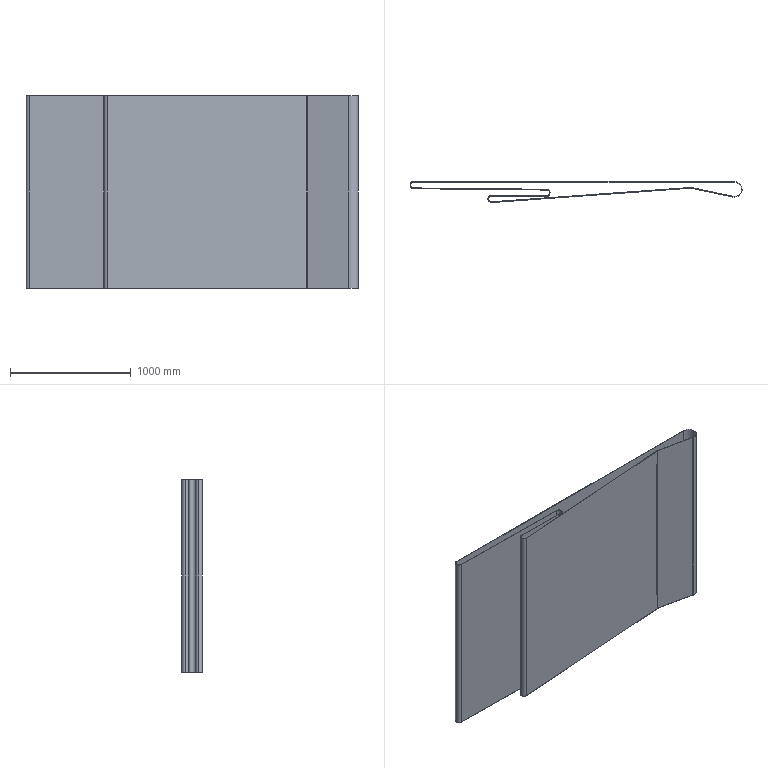Part | STEP file | Conveyor belt | 1 solid | 26 faces | box 2753 x 173 x 1600 mm | volume 42849624 mm3 | cylinder 14 | plane 12 | commonest cylinder face diameters 50 x6 58 x6 120 x1 128 x1
STEP:
#1=CARTESIAN_POINT('',(-3051.653,492.335,350.));
#2=VERTEX_POINT('',#1);
#3=CARTESIAN_POINT('',(-3080.364,521.333,350.));
#4=VERTEX_POINT('',#3);
#5=CARTESIAN_POINT('',(-3051.364,521.333,350.));
#6=DIRECTION('',(0.,0.,-1.));
#7=DIRECTION('',(-1.,0.,0.));
#8=AXIS2_PLACEMENT_3D('',#5,#6,#7);
#9=CIRCLE('',#8,29.);
#10=EDGE_CURVE('',#2,#4,#9,.T.);
#11=ORIENTED_EDGE('',*,*,#10,.T.);
#12=CARTESIAN_POINT('',(-3080.364,521.333,-1250.));
#13=VERTEX_POINT('',#12);
#14=CARTESIAN_POINT('',(-3080.364,521.333,350.));
#15=DIRECTION('',(0.,0.,-1.));
#16=VECTOR('',#15,1000.);
#17=LINE('',#14,#16);
#18=EDGE_CURVE('',#4,#13,#17,.T.);
#19=ORIENTED_EDGE('',*,*,#18,.T.);
#20=CARTESIAN_POINT('',(-3051.653,492.335,-1250.));
#21=VERTEX_POINT('',#20);
#22=CARTESIAN_POINT('',(-3051.364,521.333,-1250.));
#23=DIRECTION('',(0.,0.,-1.));
#24=DIRECTION('',(-1.,0.,0.));
#25=AXIS2_PLACEMENT_3D('',#22,#23,#24);
#26=CIRCLE('',#25,29.);
#27=EDGE_CURVE('',#21,#13,#26,.T.);
#28=ORIENTED_EDGE('',*,*,#27,.F.);
#29=CARTESIAN_POINT('',(-3051.653,492.335,350.));
#30=DIRECTION('',(0.,0.,1.));
#31=VECTOR('',#30,1000.);
#32=LINE('',#29,#31);
#33=EDGE_CURVE('',#21,#2,#32,.T.);
#34=ORIENTED_EDGE('',*,*,#33,.T.);
#35=EDGE_LOOP('',(#11,#19,#28,#34));
#36=FACE_OUTER_BOUND('',#35,.T.);
#37=CARTESIAN_POINT('',(-3051.364,521.333,350.));
#38=DIRECTION('',(0.,0.,-1.));
#39=DIRECTION('',(-1.,0.,0.));
#40=AXIS2_PLACEMENT_3D('',#37,#38,#39);
#41=CYLINDRICAL_SURFACE('',#40,29.);
#42=ADVANCED_FACE('',(#36),#41,.T.);
#43=CARTESIAN_POINT('',(-3076.364,521.333,350.));
#44=VERTEX_POINT('',#43);
#45=CARTESIAN_POINT('',(-3051.364,546.333,350.));
#46=VERTEX_POINT('',#45);
#47=CARTESIAN_POINT('',(-3051.364,521.333,350.));
#48=DIRECTION('',(0.,0.,-1.));
#49=DIRECTION('',(-1.,0.,0.));
#50=AXIS2_PLACEMENT_3D('',#47,#48,#49);
#51=CIRCLE('',#50,25.);
#52=EDGE_CURVE('',#44,#46,#51,.T.);
#53=ORIENTED_EDGE('',*,*,#52,.F.);
#54=CARTESIAN_POINT('',(-3076.364,521.333,-1250.));
#55=VERTEX_POINT('',#54);
#56=CARTESIAN_POINT('',(-3076.364,521.333,350.));
#57=DIRECTION('',(0.,0.,-1.));
#58=VECTOR('',#57,1000.);
#59=LINE('',#56,#58);
#60=EDGE_CURVE('',#44,#55,#59,.T.);
#61=ORIENTED_EDGE('',*,*,#60,.T.);
#62=CARTESIAN_POINT('',(-3051.364,546.333,-1250.));
#63=VERTEX_POINT('',#62);
#64=CARTESIAN_POINT('',(-3051.364,521.333,-1250.));
#65=DIRECTION('',(0.,0.,-1.));
#66=DIRECTION('',(-1.,0.,0.));
#67=AXIS2_PLACEMENT_3D('',#64,#65,#66);
#68=CIRCLE('',#67,25.);
#69=EDGE_CURVE('',#55,#63,#68,.T.);
#70=ORIENTED_EDGE('',*,*,#69,.T.);
#71=CARTESIAN_POINT('',(-3051.364,546.333,350.));
#72=DIRECTION('',(0.,0.,-1.));
#73=VECTOR('',#72,1000.);
#74=LINE('',#71,#73);
#75=EDGE_CURVE('',#46,#63,#74,.T.);
#76=ORIENTED_EDGE('',*,*,#75,.F.);
#77=EDGE_LOOP('',(#53,#61,#70,#76));
#78=FACE_OUTER_BOUND('',#77,.T.);
#79=CARTESIAN_POINT('',(-3051.364,521.333,350.));
#80=DIRECTION('',(0.,0.,-1.));
#81=DIRECTION('',(-1.,0.,0.));
#82=AXIS2_PLACEMENT_3D('',#79,#80,#81);
#83=CYLINDRICAL_SURFACE('',#82,25.);
#84=ADVANCED_FACE('',(#78),#83,.F.);
#85=CARTESIAN_POINT('',(-2430.364,406.333,350.));
#86=VERTEX_POINT('',#85);
#87=CARTESIAN_POINT('',(-2405.145,431.332,350.));
#88=VERTEX_POINT('',#87);
#89=CARTESIAN_POINT('',(-2405.364,406.333,350.));
#90=DIRECTION('',(0.,0.,-1.));
#91=DIRECTION('',(-1.,0.,0.));
#92=AXIS2_PLACEMENT_3D('',#89,#90,#91);
#93=CIRCLE('',#92,25.);
#94=EDGE_CURVE('',#86,#88,#93,.T.);
#95=ORIENTED_EDGE('',*,*,#94,.F.);
#96=CARTESIAN_POINT('',(-2430.364,406.333,-1250.));
#97=VERTEX_POINT('',#96);
#98=CARTESIAN_POINT('',(-2430.364,406.333,350.));
#99=DIRECTION('',(0.,0.,-1.));
#100=VECTOR('',#99,1000.);
#101=LINE('',#98,#100);
#102=EDGE_CURVE('',#86,#97,#101,.T.);
#103=ORIENTED_EDGE('',*,*,#102,.T.);
#104=CARTESIAN_POINT('',(-2405.145,431.332,-1250.));
#105=VERTEX_POINT('',#104);
#106=CARTESIAN_POINT('',(-2405.364,406.333,-1250.));
#107=DIRECTION('',(0.,0.,-1.));
#108=DIRECTION('',(-1.,0.,0.));
#109=AXIS2_PLACEMENT_3D('',#106,#107,#108);
#110=CIRCLE('',#109,25.);
#111=EDGE_CURVE('',#97,#105,#110,.T.);
#112=ORIENTED_EDGE('',*,*,#111,.T.);
#113=CARTESIAN_POINT('',(-2405.145,431.332,350.));
#114=DIRECTION('',(0.,0.,-1.));
#115=VECTOR('',#114,1000.);
#116=LINE('',#113,#115);
#117=EDGE_CURVE('',#88,#105,#116,.T.);
#118=ORIENTED_EDGE('',*,*,#117,.F.);
#119=EDGE_LOOP('',(#95,#103,#112,#118));
#120=FACE_OUTER_BOUND('',#119,.T.);
#121=CARTESIAN_POINT('',(-2405.364,406.333,350.));
#122=DIRECTION('',(0.,0.,-1.));
#123=DIRECTION('',(-1.,0.,0.));
#124=AXIS2_PLACEMENT_3D('',#121,#122,#123);
#125=CYLINDRICAL_SURFACE('',#124,25.);
#126=ADVANCED_FACE('',(#120),#125,.F.);
#127=CARTESIAN_POINT('',(-2434.364,406.333,350.));
#128=VERTEX_POINT('',#127);
#129=CARTESIAN_POINT('',(-2403.281,377.408,350.));
#130=VERTEX_POINT('',#129);
#131=CARTESIAN_POINT('',(-2405.364,406.333,350.));
#132=DIRECTION('',(0.,0.,1.));
#133=DIRECTION('',(-1.,0.,0.));
#134=AXIS2_PLACEMENT_3D('',#131,#132,#133);
#135=CIRCLE('',#134,29.);
#136=EDGE_CURVE('',#128,#130,#135,.T.);
#137=ORIENTED_EDGE('',*,*,#136,.F.);
#138=CARTESIAN_POINT('',(-2434.364,406.333,-1250.));
#139=VERTEX_POINT('',#138);
#140=CARTESIAN_POINT('',(-2434.364,406.333,350.));
#141=DIRECTION('',(0.,0.,-1.));
#142=VECTOR('',#141,1000.);
#143=LINE('',#140,#142);
#144=EDGE_CURVE('',#128,#139,#143,.T.);
#145=ORIENTED_EDGE('',*,*,#144,.T.);
#146=CARTESIAN_POINT('',(-2403.281,377.408,-1250.));
#147=VERTEX_POINT('',#146);
#148=CARTESIAN_POINT('',(-2405.364,406.333,-1250.));
#149=DIRECTION('',(0.,0.,-1.));
#150=DIRECTION('',(-1.,0.,0.));
#151=AXIS2_PLACEMENT_3D('',#148,#149,#150);
#152=CIRCLE('',#151,29.);
#153=EDGE_CURVE('',#147,#139,#152,.T.);
#154=ORIENTED_EDGE('',*,*,#153,.F.);
#155=CARTESIAN_POINT('',(-2403.281,377.408,350.));
#156=DIRECTION('',(0.,0.,1.));
#157=VECTOR('',#156,1000.);
#158=LINE('',#155,#157);
#159=EDGE_CURVE('',#147,#130,#158,.T.);
#160=ORIENTED_EDGE('',*,*,#159,.T.);
#161=EDGE_LOOP('',(#137,#145,#154,#160));
#162=FACE_OUTER_BOUND('',#161,.T.);
#163=CARTESIAN_POINT('',(-2405.364,406.333,350.));
#164=DIRECTION('',(0.,0.,-1.));
#165=DIRECTION('',(-1.,0.,0.));
#166=AXIS2_PLACEMENT_3D('',#163,#164,#165);
#167=CYLINDRICAL_SURFACE('',#166,29.);
#168=ADVANCED_FACE('',(#162),#167,.T.);
#169=CARTESIAN_POINT('',(-3051.364,550.333,350.));
#170=VERTEX_POINT('',#169);
#171=CARTESIAN_POINT('',(-3051.364,550.333,-1250.));
#172=VERTEX_POINT('',#171);
#173=CARTESIAN_POINT('',(-3051.364,550.333,350.));
#174=DIRECTION('',(0.,0.,-1.));
#175=VECTOR('',#174,1000.);
#176=LINE('',#173,#175);
#177=EDGE_CURVE('',#170,#172,#176,.T.);
#178=ORIENTED_EDGE('',*,*,#177,.F.);
#179=CARTESIAN_POINT('',(-391.364,550.333,350.));
#180=VERTEX_POINT('',#179);
#181=CARTESIAN_POINT('',(-391.364,550.333,350.));
#182=DIRECTION('',(-1.,0.,0.));
#183=VECTOR('',#182,1000.);
#184=LINE('',#181,#183);
#185=EDGE_CURVE('',#180,#170,#184,.T.);
#186=ORIENTED_EDGE('',*,*,#185,.F.);
#187=CARTESIAN_POINT('',(-391.364,550.333,-1250.));
#188=VERTEX_POINT('',#187);
#189=CARTESIAN_POINT('',(-391.364,550.333,350.));
#190=DIRECTION('',(0.,0.,1.));
#191=VECTOR('',#190,1000.);
#192=LINE('',#189,#191);
#193=EDGE_CURVE('',#188,#180,#192,.T.);
#194=ORIENTED_EDGE('',*,*,#193,.F.);
#195=CARTESIAN_POINT('',(-3051.364,550.333,-1250.));
#196=DIRECTION('',(1.,0.,0.));
#197=VECTOR('',#196,1000.);
#198=LINE('',#195,#197);
#199=EDGE_CURVE('',#172,#188,#198,.T.);
#200=ORIENTED_EDGE('',*,*,#199,.F.);
#201=EDGE_LOOP('',(#178,#186,#194,#200));
#202=FACE_OUTER_BOUND('',#201,.T.);
#203=CARTESIAN_POINT('',(-391.364,550.333,350.));
#204=DIRECTION('',(0.,-1.,0.));
#205=DIRECTION('',(1.,0.,0.));
#206=AXIS2_PLACEMENT_3D('',#203,#204,#205);
#207=PLANE('',#206);
#208=ADVANCED_FACE('',(#202),#207,.F.);
#209=ORIENTED_EDGE('',*,*,#18,.F.);
#210=CARTESIAN_POINT('',(-3051.364,521.333,350.));
#211=DIRECTION('',(0.,0.,-1.));
#212=DIRECTION('',(-1.,0.,0.));
#213=AXIS2_PLACEMENT_3D('',#210,#211,#212);
#214=CIRCLE('',#213,29.);
#215=EDGE_CURVE('',#4,#170,#214,.T.);
#216=ORIENTED_EDGE('',*,*,#215,.T.);
#217=ORIENTED_EDGE('',*,*,#177,.T.);
#218=CARTESIAN_POINT('',(-3051.364,521.333,-1250.));
#219=DIRECTION('',(0.,0.,-1.));
#220=DIRECTION('',(-1.,0.,0.));
#221=AXIS2_PLACEMENT_3D('',#218,#219,#220);
#222=CIRCLE('',#221,29.);
#223=EDGE_CURVE('',#13,#172,#222,.T.);
#224=ORIENTED_EDGE('',*,*,#223,.F.);
#225=EDGE_LOOP('',(#209,#216,#217,#224));
#226=FACE_OUTER_BOUND('',#225,.T.);
#227=CARTESIAN_POINT('',(-3051.364,521.333,350.));
#228=DIRECTION('',(0.,0.,-1.));
#229=DIRECTION('',(-1.,0.,0.));
#230=AXIS2_PLACEMENT_3D('',#227,#228,#229);
#231=CYLINDRICAL_SURFACE('',#230,29.);
#232=ADVANCED_FACE('',(#226),#231,.T.);
#233=CARTESIAN_POINT('',(-391.364,546.333,350.));
#234=VERTEX_POINT('',#233);
#235=CARTESIAN_POINT('',(-2405.364,546.333,350.));
#236=DIRECTION('',(1.,0.,0.));
#237=VECTOR('',#236,1000.);
#238=LINE('',#235,#237);
#239=EDGE_CURVE('',#46,#234,#238,.T.);
#240=ORIENTED_EDGE('',*,*,#239,.T.);
#241=CARTESIAN_POINT('',(-403.751,427.626,350.));
#242=VERTEX_POINT('',#241);
#243=CARTESIAN_POINT('',(-391.364,486.333,350.));
#244=DIRECTION('',(0.,0.,-1.));
#245=DIRECTION('',(-1.,0.,0.));
#246=AXIS2_PLACEMENT_3D('',#243,#244,#245);
#247=CIRCLE('',#246,60.);
#248=EDGE_CURVE('',#234,#242,#247,.T.);
#249=ORIENTED_EDGE('',*,*,#248,.T.);
#250=CARTESIAN_POINT('',(-745.377,499.709,350.));
#251=VERTEX_POINT('',#250);
#252=CARTESIAN_POINT('',(-403.751,427.626,350.));
#253=DIRECTION('',(-0.9785,0.2065,0.));
#254=VECTOR('',#253,1000.);
#255=LINE('',#252,#254);
#256=EDGE_CURVE('',#242,#251,#255,.T.);
#257=ORIENTED_EDGE('',*,*,#256,.T.);
#258=CARTESIAN_POINT('',(-753.448,500.258,350.));
#259=VERTEX_POINT('',#258);
#260=CARTESIAN_POINT('',(-751.364,471.333,350.));
#261=DIRECTION('',(0.,0.,1.));
#262=DIRECTION('',(-1.,0.,0.));
#263=AXIS2_PLACEMENT_3D('',#260,#261,#262);
#264=CIRCLE('',#263,29.);
#265=EDGE_CURVE('',#251,#259,#264,.T.);
#266=ORIENTED_EDGE('',*,*,#265,.T.);
#267=CARTESIAN_POINT('',(-2403.568,381.398,350.));
#268=VERTEX_POINT('',#267);
#269=CARTESIAN_POINT('',(-753.448,500.258,350.));
#270=DIRECTION('',(-0.9974,-0.07185,0.));
#271=VECTOR('',#270,1000.);
#272=LINE('',#269,#271);
#273=EDGE_CURVE('',#259,#268,#272,.T.);
#274=ORIENTED_EDGE('',*,*,#273,.T.);
#275=CARTESIAN_POINT('',(-2405.364,406.333,350.));
#276=DIRECTION('',(0.,0.,-1.));
#277=DIRECTION('',(-1.,0.,0.));
#278=AXIS2_PLACEMENT_3D('',#275,#276,#277);
#279=CIRCLE('',#278,25.);
#280=EDGE_CURVE('',#268,#86,#279,.T.);
#281=ORIENTED_EDGE('',*,*,#280,.T.);
#282=ORIENTED_EDGE('',*,*,#94,.T.);
#283=CARTESIAN_POINT('',(-1948.618,427.334,350.));
#284=VERTEX_POINT('',#283);
#285=CARTESIAN_POINT('',(-2405.145,431.332,350.));
#286=DIRECTION('',(1.,-0.008757,0.));
#287=VECTOR('',#286,1000.);
#288=LINE('',#285,#287);
#289=EDGE_CURVE('',#88,#284,#288,.T.);
#290=ORIENTED_EDGE('',*,*,#289,.T.);
#291=CARTESIAN_POINT('',(-1948.075,485.332,350.));
#292=VERTEX_POINT('',#291);
#293=CARTESIAN_POINT('',(-1948.364,456.333,350.));
#294=DIRECTION('',(0.,0.,1.));
#295=DIRECTION('',(-1.,0.,0.));
#296=AXIS2_PLACEMENT_3D('',#293,#294,#295);
#297=CIRCLE('',#296,29.);
#298=EDGE_CURVE('',#284,#292,#297,.T.);
#299=ORIENTED_EDGE('',*,*,#298,.T.);
#300=CARTESIAN_POINT('',(-3051.613,496.335,350.));
#301=VERTEX_POINT('',#300);
#302=CARTESIAN_POINT('',(-1948.075,485.332,350.));
#303=DIRECTION('',(-1.,0.00997,0.));
#304=VECTOR('',#303,1000.);
#305=LINE('',#302,#304);
#306=EDGE_CURVE('',#292,#301,#305,.T.);
#307=ORIENTED_EDGE('',*,*,#306,.T.);
#308=CARTESIAN_POINT('',(-3051.364,521.333,350.));
#309=DIRECTION('',(0.,0.,-1.));
#310=DIRECTION('',(-1.,0.,0.));
#311=AXIS2_PLACEMENT_3D('',#308,#309,#310);
#312=CIRCLE('',#311,25.);
#313=EDGE_CURVE('',#301,#44,#312,.T.);
#314=ORIENTED_EDGE('',*,*,#313,.T.);
#315=ORIENTED_EDGE('',*,*,#52,.T.);
#316=EDGE_LOOP('',(#240,#249,#257,#266,#274,#281,#282,#290,#299,#307,#314,#315));
#317=FACE_BOUND('',#316,.T.);
#318=CARTESIAN_POINT('',(-1948.115,481.332,350.));
#319=VERTEX_POINT('',#318);
#320=CARTESIAN_POINT('',(-1948.583,431.334,350.));
#321=VERTEX_POINT('',#320);
#322=CARTESIAN_POINT('',(-1948.364,456.333,350.));
#323=DIRECTION('',(0.,0.,-1.));
#324=DIRECTION('',(-1.,0.,0.));
#325=AXIS2_PLACEMENT_3D('',#322,#323,#324);
#326=CIRCLE('',#325,25.);
#327=EDGE_CURVE('',#319,#321,#326,.T.);
#328=ORIENTED_EDGE('',*,*,#327,.T.);
#329=CARTESIAN_POINT('',(-2405.11,435.332,350.));
#330=VERTEX_POINT('',#329);
#331=CARTESIAN_POINT('',(-1948.583,431.334,350.));
#332=DIRECTION('',(-1.,0.008757,0.));
#333=VECTOR('',#332,1000.);
#334=LINE('',#331,#333);
#335=EDGE_CURVE('',#321,#330,#334,.T.);
#336=ORIENTED_EDGE('',*,*,#335,.T.);
#337=CARTESIAN_POINT('',(-2405.364,406.333,350.));
#338=DIRECTION('',(0.,0.,1.));
#339=DIRECTION('',(-1.,0.,0.));
#340=AXIS2_PLACEMENT_3D('',#337,#338,#339);
#341=CIRCLE('',#340,29.);
#342=EDGE_CURVE('',#330,#128,#341,.T.);
#343=ORIENTED_EDGE('',*,*,#342,.T.);
#344=ORIENTED_EDGE('',*,*,#136,.T.);
#345=CARTESIAN_POINT('',(-753.16,496.269,350.));
#346=VERTEX_POINT('',#345);
#347=CARTESIAN_POINT('',(-2403.281,377.408,350.));
#348=DIRECTION('',(0.9974,0.07185,0.));
#349=VECTOR('',#348,1000.);
#350=LINE('',#347,#349);
#351=EDGE_CURVE('',#130,#346,#350,.T.);
#352=ORIENTED_EDGE('',*,*,#351,.T.);
#353=CARTESIAN_POINT('',(-746.203,495.795,350.));
#354=VERTEX_POINT('',#353);
#355=CARTESIAN_POINT('',(-751.364,471.333,350.));
#356=DIRECTION('',(0.,0.,-1.));
#357=DIRECTION('',(-1.,0.,0.));
#358=AXIS2_PLACEMENT_3D('',#355,#356,#357);
#359=CIRCLE('',#358,25.);
#360=EDGE_CURVE('',#346,#354,#359,.T.);
#361=ORIENTED_EDGE('',*,*,#360,.T.);
#362=CARTESIAN_POINT('',(-404.577,423.712,350.));
#363=VERTEX_POINT('',#362);
#364=CARTESIAN_POINT('',(-746.203,495.795,350.));
#365=DIRECTION('',(0.9785,-0.2065,0.));
#366=VECTOR('',#365,1000.);
#367=LINE('',#364,#366);
#368=EDGE_CURVE('',#354,#363,#367,.T.);
#369=ORIENTED_EDGE('',*,*,#368,.T.);
#370=CARTESIAN_POINT('',(-391.364,486.333,350.));
#371=DIRECTION('',(0.,0.,1.));
#372=DIRECTION('',(-1.,0.,0.));
#373=AXIS2_PLACEMENT_3D('',#370,#371,#372);
#374=CIRCLE('',#373,64.);
#375=EDGE_CURVE('',#363,#180,#374,.T.);
#376=ORIENTED_EDGE('',*,*,#375,.T.);
#377=ORIENTED_EDGE('',*,*,#185,.T.);
#378=ORIENTED_EDGE('',*,*,#215,.F.);
#379=ORIENTED_EDGE('',*,*,#10,.F.);
#380=CARTESIAN_POINT('',(-3051.653,492.335,350.));
#381=DIRECTION('',(1.,-0.00997,0.));
#382=VECTOR('',#381,1000.);
#383=LINE('',#380,#382);
#384=EDGE_CURVE('',#2,#319,#383,.T.);
#385=ORIENTED_EDGE('',*,*,#384,.T.);
#386=EDGE_LOOP('',(#328,#336,#343,#344,#352,#361,#369,#376,#377,#378,#379,#385));
#387=FACE_OUTER_BOUND('',#386,.T.);
#388=CARTESIAN_POINT('',(-2405.364,406.333,350.));
#389=DIRECTION('',(0.,0.,1.));
#390=DIRECTION('',(1.,0.,0.));
#391=AXIS2_PLACEMENT_3D('',#388,#389,#390);
#392=PLANE('',#391);
#393=ADVANCED_FACE('',(#317,#387),#392,.T.);
#394=ORIENTED_EDGE('',*,*,#375,.F.);
#395=CARTESIAN_POINT('',(-404.577,423.712,-1250.));
#396=VERTEX_POINT('',#395);
#397=CARTESIAN_POINT('',(-404.577,423.712,350.));
#398=DIRECTION('',(0.,0.,-1.));
#399=VECTOR('',#398,1000.);
#400=LINE('',#397,#399);
#401=EDGE_CURVE('',#363,#396,#400,.T.);
#402=ORIENTED_EDGE('',*,*,#401,.T.);
#403=CARTESIAN_POINT('',(-391.364,486.333,-1250.));
#404=DIRECTION('',(0.,0.,-1.));
#405=DIRECTION('',(-1.,0.,0.));
#406=AXIS2_PLACEMENT_3D('',#403,#404,#405);
#407=CIRCLE('',#406,64.);
#408=EDGE_CURVE('',#188,#396,#407,.T.);
#409=ORIENTED_EDGE('',*,*,#408,.F.);
#410=ORIENTED_EDGE('',*,*,#193,.T.);
#411=EDGE_LOOP('',(#394,#402,#409,#410));
#412=FACE_OUTER_BOUND('',#411,.T.);
#413=CARTESIAN_POINT('',(-391.364,486.333,350.));
#414=DIRECTION('',(0.,0.,-1.));
#415=DIRECTION('',(-1.,0.,0.));
#416=AXIS2_PLACEMENT_3D('',#413,#414,#415);
#417=CYLINDRICAL_SURFACE('',#416,64.);
#418=ADVANCED_FACE('',(#412),#417,.T.);
#419=ORIENTED_EDGE('',*,*,#265,.F.);
#420=CARTESIAN_POINT('',(-745.377,499.709,-1250.));
#421=VERTEX_POINT('',#420);
#422=CARTESIAN_POINT('',(-745.377,499.709,350.));
#423=DIRECTION('',(0.,0.,-1.));
#424=VECTOR('',#423,1000.);
#425=LINE('',#422,#424);
#426=EDGE_CURVE('',#251,#421,#425,.T.);
#427=ORIENTED_EDGE('',*,*,#426,.T.);
#428=CARTESIAN_POINT('',(-753.448,500.258,-1250.));
#429=VERTEX_POINT('',#428);
#430=CARTESIAN_POINT('',(-751.364,471.333,-1250.));
#431=DIRECTION('',(0.,0.,1.));
#432=DIRECTION('',(-1.,0.,0.));
#433=AXIS2_PLACEMENT_3D('',#430,#431,#432);
#434=CIRCLE('',#433,29.);
#435=EDGE_CURVE('',#421,#429,#434,.T.);
#436=ORIENTED_EDGE('',*,*,#435,.T.);
#437=CARTESIAN_POINT('',(-753.448,500.258,350.));
#438=DIRECTION('',(0.,0.,1.));
#439=VECTOR('',#438,1000.);
#440=LINE('',#437,#439);
#441=EDGE_CURVE('',#429,#259,#440,.T.);
#442=ORIENTED_EDGE('',*,*,#441,.T.);
#443=EDGE_LOOP('',(#419,#427,#436,#442));
#444=FACE_OUTER_BOUND('',#443,.T.);
#445=CARTESIAN_POINT('',(-751.364,471.333,350.));
#446=DIRECTION('',(0.,0.,-1.));
#447=DIRECTION('',(-1.,0.,0.));
#448=AXIS2_PLACEMENT_3D('',#445,#446,#447);
#449=CYLINDRICAL_SURFACE('',#448,29.);
#450=ADVANCED_FACE('',(#444),#449,.T.);
#451=ORIENTED_EDGE('',*,*,#256,.F.);
#452=CARTESIAN_POINT('',(-403.751,427.626,-1250.));
#453=VERTEX_POINT('',#452);
#454=CARTESIAN_POINT('',(-403.751,427.626,350.));
#455=DIRECTION('',(0.,0.,-1.));
#456=VECTOR('',#455,1000.);
#457=LINE('',#454,#456);
#458=EDGE_CURVE('',#242,#453,#457,.T.);
#459=ORIENTED_EDGE('',*,*,#458,.T.);
#460=CARTESIAN_POINT('',(-403.751,427.626,-1250.));
#461=DIRECTION('',(-0.9785,0.2065,0.));
#462=VECTOR('',#461,1000.);
#463=LINE('',#460,#462);
#464=EDGE_CURVE('',#453,#421,#463,.T.);
#465=ORIENTED_EDGE('',*,*,#464,.T.);
#466=ORIENTED_EDGE('',*,*,#426,.F.);
#467=EDGE_LOOP('',(#451,#459,#465,#466));
#468=FACE_OUTER_BOUND('',#467,.T.);
#469=CARTESIAN_POINT('',(-745.377,499.709,350.));
#470=DIRECTION('',(0.2065,0.9785,0.));
#471=DIRECTION('',(-0.9785,0.2065,0.));
#472=AXIS2_PLACEMENT_3D('',#469,#470,#471);
#473=PLANE('',#472);
#474=ADVANCED_FACE('',(#468),#473,.T.);
#475=ORIENTED_EDGE('',*,*,#458,.F.);
#476=ORIENTED_EDGE('',*,*,#248,.F.);
#477=CARTESIAN_POINT('',(-391.364,546.333,-1250.));
#478=VERTEX_POINT('',#477);
#479=CARTESIAN_POINT('',(-391.364,546.333,350.));
#480=DIRECTION('',(0.,0.,1.));
#481=VECTOR('',#480,1000.);
#482=LINE('',#479,#481);
#483=EDGE_CURVE('',#478,#234,#482,.T.);
#484=ORIENTED_EDGE('',*,*,#483,.F.);
#485=CARTESIAN_POINT('',(-391.364,486.333,-1250.));
#486=DIRECTION('',(0.,0.,-1.));
#487=DIRECTION('',(-1.,0.,0.));
#488=AXIS2_PLACEMENT_3D('',#485,#486,#487);
#489=CIRCLE('',#488,60.);
#490=EDGE_CURVE('',#478,#453,#489,.T.);
#491=ORIENTED_EDGE('',*,*,#490,.T.);
#492=EDGE_LOOP('',(#475,#476,#484,#491));
#493=FACE_OUTER_BOUND('',#492,.T.);
#494=CARTESIAN_POINT('',(-391.364,486.333,350.));
#495=DIRECTION('',(0.,0.,-1.));
#496=DIRECTION('',(-1.,0.,0.));
#497=AXIS2_PLACEMENT_3D('',#494,#495,#496);
#498=CYLINDRICAL_SURFACE('',#497,60.);
#499=ADVANCED_FACE('',(#493),#498,.F.);
#500=ORIENTED_EDGE('',*,*,#239,.F.);
#501=ORIENTED_EDGE('',*,*,#75,.T.);
#502=CARTESIAN_POINT('',(-3051.364,546.333,-1250.));
#503=DIRECTION('',(1.,0.,0.));
#504=VECTOR('',#503,1000.);
#505=LINE('',#502,#504);
#506=EDGE_CURVE('',#63,#478,#505,.T.);
#507=ORIENTED_EDGE('',*,*,#506,.T.);
#508=ORIENTED_EDGE('',*,*,#483,.T.);
#509=EDGE_LOOP('',(#500,#501,#507,#508));
#510=FACE_OUTER_BOUND('',#509,.T.);
#511=CARTESIAN_POINT('',(-3051.364,546.333,350.));
#512=DIRECTION('',(0.,-1.,0.));
#513=DIRECTION('',(1.,0.,0.));
#514=AXIS2_PLACEMENT_3D('',#511,#512,#513);
#515=PLANE('',#514);
#516=ADVANCED_FACE('',(#510),#515,.T.);
#517=ORIENTED_EDGE('',*,*,#60,.F.);
#518=ORIENTED_EDGE('',*,*,#313,.F.);
#519=CARTESIAN_POINT('',(-3051.613,496.335,-1250.));
#520=VERTEX_POINT('',#519);
#521=CARTESIAN_POINT('',(-3051.613,496.335,350.));
#522=DIRECTION('',(0.,0.,1.));
#523=VECTOR('',#522,1000.);
#524=LINE('',#521,#523);
#525=EDGE_CURVE('',#520,#301,#524,.T.);
#526=ORIENTED_EDGE('',*,*,#525,.F.);
#527=CARTESIAN_POINT('',(-3051.364,521.333,-1250.));
#528=DIRECTION('',(0.,0.,-1.));
#529=DIRECTION('',(-1.,0.,0.));
#530=AXIS2_PLACEMENT_3D('',#527,#528,#529);
#531=CIRCLE('',#530,25.);
#532=EDGE_CURVE('',#520,#55,#531,.T.);
#533=ORIENTED_EDGE('',*,*,#532,.T.);
#534=EDGE_LOOP('',(#517,#518,#526,#533));
#535=FACE_OUTER_BOUND('',#534,.T.);
#536=CARTESIAN_POINT('',(-3051.364,521.333,350.));
#537=DIRECTION('',(0.,0.,-1.));
#538=DIRECTION('',(-1.,0.,0.));
#539=AXIS2_PLACEMENT_3D('',#536,#537,#538);
#540=CYLINDRICAL_SURFACE('',#539,25.);
#541=ADVANCED_FACE('',(#535),#540,.F.);
#542=ORIENTED_EDGE('',*,*,#306,.F.);
#543=CARTESIAN_POINT('',(-1948.075,485.332,-1250.));
#544=VERTEX_POINT('',#543);
#545=CARTESIAN_POINT('',(-1948.075,485.332,350.));
#546=DIRECTION('',(0.,0.,-1.));
#547=VECTOR('',#546,1000.);
#548=LINE('',#545,#547);
#549=EDGE_CURVE('',#292,#544,#548,.T.);
#550=ORIENTED_EDGE('',*,*,#549,.T.);
#551=CARTESIAN_POINT('',(-1948.075,485.332,-1250.));
#552=DIRECTION('',(-1.,0.00997,0.));
#553=VECTOR('',#552,1000.);
#554=LINE('',#551,#553);
#555=EDGE_CURVE('',#544,#520,#554,.T.);
#556=ORIENTED_EDGE('',*,*,#555,.T.);
#557=ORIENTED_EDGE('',*,*,#525,.T.);
#558=EDGE_LOOP('',(#542,#550,#556,#557));
#559=FACE_OUTER_BOUND('',#558,.T.);
#560=CARTESIAN_POINT('',(-3051.613,496.335,350.));
#561=DIRECTION('',(0.00997,1.,0.));
#562=DIRECTION('',(-1.,0.00997,0.));
#563=AXIS2_PLACEMENT_3D('',#560,#561,#562);
#564=PLANE('',#563);
#565=ADVANCED_FACE('',(#559),#564,.T.);
#566=ORIENTED_EDGE('',*,*,#298,.F.);
#567=CARTESIAN_POINT('',(-1948.618,427.334,-1250.));
#568=VERTEX_POINT('',#567);
#569=CARTESIAN_POINT('',(-1948.618,427.334,350.));
#570=DIRECTION('',(0.,0.,-1.));
#571=VECTOR('',#570,1000.);
#572=LINE('',#569,#571);
#573=EDGE_CURVE('',#284,#568,#572,.T.);
#574=ORIENTED_EDGE('',*,*,#573,.T.);
#575=CARTESIAN_POINT('',(-1948.364,456.333,-1250.));
#576=DIRECTION('',(0.,0.,1.));
#577=DIRECTION('',(-1.,0.,0.));
#578=AXIS2_PLACEMENT_3D('',#575,#576,#577);
#579=CIRCLE('',#578,29.);
#580=EDGE_CURVE('',#568,#544,#579,.T.);
#581=ORIENTED_EDGE('',*,*,#580,.T.);
#582=ORIENTED_EDGE('',*,*,#549,.F.);
#583=EDGE_LOOP('',(#566,#574,#581,#582));
#584=FACE_OUTER_BOUND('',#583,.T.);
#585=CARTESIAN_POINT('',(-1948.364,456.333,350.));
#586=DIRECTION('',(0.,0.,-1.));
#587=DIRECTION('',(-1.,0.,0.));
#588=AXIS2_PLACEMENT_3D('',#585,#586,#587);
#589=CYLINDRICAL_SURFACE('',#588,29.);
#590=ADVANCED_FACE('',(#584),#589,.T.);
#591=ORIENTED_EDGE('',*,*,#289,.F.);
#592=ORIENTED_EDGE('',*,*,#117,.T.);
#593=CARTESIAN_POINT('',(-2405.145,431.332,-1250.));
#594=DIRECTION('',(1.,-0.008757,0.));
#595=VECTOR('',#594,1000.);
#596=LINE('',#593,#595);
#597=EDGE_CURVE('',#105,#568,#596,.T.);
#598=ORIENTED_EDGE('',*,*,#597,.T.);
#599=ORIENTED_EDGE('',*,*,#573,.F.);
#600=EDGE_LOOP('',(#591,#592,#598,#599));
#601=FACE_OUTER_BOUND('',#600,.T.);
#602=CARTESIAN_POINT('',(-1948.618,427.334,350.));
#603=DIRECTION('',(-0.008757,-1.,0.));
#604=DIRECTION('',(1.,-0.008757,0.));
#605=AXIS2_PLACEMENT_3D('',#602,#603,#604);
#606=PLANE('',#605);
#607=ADVANCED_FACE('',(#601),#606,.T.);
#608=ORIENTED_EDGE('',*,*,#102,.F.);
#609=ORIENTED_EDGE('',*,*,#280,.F.);
#610=CARTESIAN_POINT('',(-2403.568,381.398,-1250.));
#611=VERTEX_POINT('',#610);
#612=CARTESIAN_POINT('',(-2403.568,381.398,350.));
#613=DIRECTION('',(0.,0.,1.));
#614=VECTOR('',#613,1000.);
#615=LINE('',#612,#614);
#616=EDGE_CURVE('',#611,#268,#615,.T.);
#617=ORIENTED_EDGE('',*,*,#616,.F.);
#618=CARTESIAN_POINT('',(-2405.364,406.333,-1250.));
#619=DIRECTION('',(0.,0.,-1.));
#620=DIRECTION('',(-1.,0.,0.));
#621=AXIS2_PLACEMENT_3D('',#618,#619,#620);
#622=CIRCLE('',#621,25.);
#623=EDGE_CURVE('',#611,#97,#622,.T.);
#624=ORIENTED_EDGE('',*,*,#623,.T.);
#625=EDGE_LOOP('',(#608,#609,#617,#624));
#626=FACE_OUTER_BOUND('',#625,.T.);
#627=CARTESIAN_POINT('',(-2405.364,406.333,350.));
#628=DIRECTION('',(0.,0.,-1.));
#629=DIRECTION('',(-1.,0.,0.));
#630=AXIS2_PLACEMENT_3D('',#627,#628,#629);
#631=CYLINDRICAL_SURFACE('',#630,25.);
#632=ADVANCED_FACE('',(#626),#631,.F.);
#633=ORIENTED_EDGE('',*,*,#273,.F.);
#634=ORIENTED_EDGE('',*,*,#441,.F.);
#635=CARTESIAN_POINT('',(-753.448,500.258,-1250.));
#636=DIRECTION('',(-0.9974,-0.07185,0.));
#637=VECTOR('',#636,1000.);
#638=LINE('',#635,#637);
#639=EDGE_CURVE('',#429,#611,#638,.T.);
#640=ORIENTED_EDGE('',*,*,#639,.T.);
#641=ORIENTED_EDGE('',*,*,#616,.T.);
#642=EDGE_LOOP('',(#633,#634,#640,#641));
#643=FACE_OUTER_BOUND('',#642,.T.);
#644=CARTESIAN_POINT('',(-2403.568,381.398,350.));
#645=DIRECTION('',(-0.07185,0.9974,0.));
#646=DIRECTION('',(-0.9974,-0.07185,0.));
#647=AXIS2_PLACEMENT_3D('',#644,#645,#646);
#648=PLANE('',#647);
#649=ADVANCED_FACE('',(#643),#648,.T.);
#650=ORIENTED_EDGE('',*,*,#144,.F.);
#651=ORIENTED_EDGE('',*,*,#342,.F.);
#652=CARTESIAN_POINT('',(-2405.11,435.332,-1250.));
#653=VERTEX_POINT('',#652);
#654=CARTESIAN_POINT('',(-2405.11,435.332,350.));
#655=DIRECTION('',(0.,0.,-1.));
#656=VECTOR('',#655,1000.);
#657=LINE('',#654,#656);
#658=EDGE_CURVE('',#330,#653,#657,.T.);
#659=ORIENTED_EDGE('',*,*,#658,.T.);
#660=CARTESIAN_POINT('',(-2405.364,406.333,-1250.));
#661=DIRECTION('',(0.,0.,-1.));
#662=DIRECTION('',(-1.,0.,0.));
#663=AXIS2_PLACEMENT_3D('',#660,#661,#662);
#664=CIRCLE('',#663,29.);
#665=EDGE_CURVE('',#139,#653,#664,.T.);
#666=ORIENTED_EDGE('',*,*,#665,.F.);
#667=EDGE_LOOP('',(#650,#651,#659,#666));
#668=FACE_OUTER_BOUND('',#667,.T.);
#669=CARTESIAN_POINT('',(-2405.364,406.333,350.));
#670=DIRECTION('',(0.,0.,-1.));
#671=DIRECTION('',(-1.,0.,0.));
#672=AXIS2_PLACEMENT_3D('',#669,#670,#671);
#673=CYLINDRICAL_SURFACE('',#672,29.);
#674=ADVANCED_FACE('',(#668),#673,.T.);
#675=ORIENTED_EDGE('',*,*,#658,.F.);
#676=ORIENTED_EDGE('',*,*,#335,.F.);
#677=CARTESIAN_POINT('',(-1948.583,431.334,-1250.));
#678=VERTEX_POINT('',#677);
#679=CARTESIAN_POINT('',(-1948.583,431.334,350.));
#680=DIRECTION('',(0.,0.,1.));
#681=VECTOR('',#680,1000.);
#682=LINE('',#679,#681);
#683=EDGE_CURVE('',#678,#321,#682,.T.);
#684=ORIENTED_EDGE('',*,*,#683,.F.);
#685=CARTESIAN_POINT('',(-2405.11,435.332,-1250.));
#686=DIRECTION('',(1.,-0.008757,0.));
#687=VECTOR('',#686,1000.);
#688=LINE('',#685,#687);
#689=EDGE_CURVE('',#653,#678,#688,.T.);
#690=ORIENTED_EDGE('',*,*,#689,.F.);
#691=EDGE_LOOP('',(#675,#676,#684,#690));
#692=FACE_OUTER_BOUND('',#691,.T.);
#693=CARTESIAN_POINT('',(-2405.11,435.332,350.));
#694=DIRECTION('',(-0.008757,-1.,0.));
#695=DIRECTION('',(1.,-0.008757,0.));
#696=AXIS2_PLACEMENT_3D('',#693,#694,#695);
#697=PLANE('',#696);
#698=ADVANCED_FACE('',(#692),#697,.F.);
#699=ORIENTED_EDGE('',*,*,#683,.T.);
#700=ORIENTED_EDGE('',*,*,#327,.F.);
#701=CARTESIAN_POINT('',(-1948.115,481.332,-1250.));
#702=VERTEX_POINT('',#701);
#703=CARTESIAN_POINT('',(-1948.115,481.332,350.));
#704=DIRECTION('',(0.,0.,1.));
#705=VECTOR('',#704,1000.);
#706=LINE('',#703,#705);
#707=EDGE_CURVE('',#702,#319,#706,.T.);
#708=ORIENTED_EDGE('',*,*,#707,.F.);
#709=CARTESIAN_POINT('',(-1948.364,456.333,-1250.));
#710=DIRECTION('',(0.,0.,1.));
#711=DIRECTION('',(-1.,0.,0.));
#712=AXIS2_PLACEMENT_3D('',#709,#710,#711);
#713=CIRCLE('',#712,25.);
#714=EDGE_CURVE('',#678,#702,#713,.T.);
#715=ORIENTED_EDGE('',*,*,#714,.F.);
#716=EDGE_LOOP('',(#699,#700,#708,#715));
#717=FACE_OUTER_BOUND('',#716,.T.);
#718=CARTESIAN_POINT('',(-1948.364,456.333,350.));
#719=DIRECTION('',(0.,0.,-1.));
#720=DIRECTION('',(-1.,0.,0.));
#721=AXIS2_PLACEMENT_3D('',#718,#719,#720);
#722=CYLINDRICAL_SURFACE('',#721,25.);
#723=ADVANCED_FACE('',(#717),#722,.F.);
#724=ORIENTED_EDGE('',*,*,#707,.T.);
#725=ORIENTED_EDGE('',*,*,#384,.F.);
#726=ORIENTED_EDGE('',*,*,#33,.F.);
#727=CARTESIAN_POINT('',(-1948.115,481.332,-1250.));
#728=DIRECTION('',(-1.,0.00997,0.));
#729=VECTOR('',#728,1000.);
#730=LINE('',#727,#729);
#731=EDGE_CURVE('',#702,#21,#730,.T.);
#732=ORIENTED_EDGE('',*,*,#731,.F.);
#733=EDGE_LOOP('',(#724,#725,#726,#732));
#734=FACE_OUTER_BOUND('',#733,.T.);
#735=CARTESIAN_POINT('',(-3051.653,492.335,350.));
#736=DIRECTION('',(0.00997,1.,0.));
#737=DIRECTION('',(-1.,0.00997,0.));
#738=AXIS2_PLACEMENT_3D('',#735,#736,#737);
#739=PLANE('',#738);
#740=ADVANCED_FACE('',(#734),#739,.F.);
#741=ORIENTED_EDGE('',*,*,#401,.F.);
#742=ORIENTED_EDGE('',*,*,#368,.F.);
#743=CARTESIAN_POINT('',(-746.203,495.795,-1250.));
#744=VERTEX_POINT('',#743);
#745=CARTESIAN_POINT('',(-746.203,495.795,350.));
#746=DIRECTION('',(0.,0.,1.));
#747=VECTOR('',#746,1000.);
#748=LINE('',#745,#747);
#749=EDGE_CURVE('',#744,#354,#748,.T.);
#750=ORIENTED_EDGE('',*,*,#749,.F.);
#751=CARTESIAN_POINT('',(-404.577,423.712,-1250.));
#752=DIRECTION('',(-0.9785,0.2065,0.));
#753=VECTOR('',#752,1000.);
#754=LINE('',#751,#753);
#755=EDGE_CURVE('',#396,#744,#754,.T.);
#756=ORIENTED_EDGE('',*,*,#755,.F.);
#757=EDGE_LOOP('',(#741,#742,#750,#756));
#758=FACE_OUTER_BOUND('',#757,.T.);
#759=CARTESIAN_POINT('',(-746.203,495.795,350.));
#760=DIRECTION('',(0.2065,0.9785,0.));
#761=DIRECTION('',(-0.9785,0.2065,0.));
#762=AXIS2_PLACEMENT_3D('',#759,#760,#761);
#763=PLANE('',#762);
#764=ADVANCED_FACE('',(#758),#763,.F.);
#765=ORIENTED_EDGE('',*,*,#749,.T.);
#766=ORIENTED_EDGE('',*,*,#360,.F.);
#767=CARTESIAN_POINT('',(-753.16,496.269,-1250.));
#768=VERTEX_POINT('',#767);
#769=CARTESIAN_POINT('',(-753.16,496.269,350.));
#770=DIRECTION('',(0.,0.,1.));
#771=VECTOR('',#770,1000.);
#772=LINE('',#769,#771);
#773=EDGE_CURVE('',#768,#346,#772,.T.);
#774=ORIENTED_EDGE('',*,*,#773,.F.);
#775=CARTESIAN_POINT('',(-751.364,471.333,-1250.));
#776=DIRECTION('',(0.,0.,1.));
#777=DIRECTION('',(-1.,0.,0.));
#778=AXIS2_PLACEMENT_3D('',#775,#776,#777);
#779=CIRCLE('',#778,25.);
#780=EDGE_CURVE('',#744,#768,#779,.T.);
#781=ORIENTED_EDGE('',*,*,#780,.F.);
#782=EDGE_LOOP('',(#765,#766,#774,#781));
#783=FACE_OUTER_BOUND('',#782,.T.);
#784=CARTESIAN_POINT('',(-751.364,471.333,350.));
#785=DIRECTION('',(0.,0.,-1.));
#786=DIRECTION('',(-1.,0.,0.));
#787=AXIS2_PLACEMENT_3D('',#784,#785,#786);
#788=CYLINDRICAL_SURFACE('',#787,25.);
#789=ADVANCED_FACE('',(#783),#788,.F.);
#790=ORIENTED_EDGE('',*,*,#773,.T.);
#791=ORIENTED_EDGE('',*,*,#351,.F.);
#792=ORIENTED_EDGE('',*,*,#159,.F.);
#793=CARTESIAN_POINT('',(-753.16,496.269,-1250.));
#794=DIRECTION('',(-0.9974,-0.07185,0.));
#795=VECTOR('',#794,1000.);
#796=LINE('',#793,#795);
#797=EDGE_CURVE('',#768,#147,#796,.T.);
#798=ORIENTED_EDGE('',*,*,#797,.F.);
#799=EDGE_LOOP('',(#790,#791,#792,#798));
#800=FACE_OUTER_BOUND('',#799,.T.);
#801=CARTESIAN_POINT('',(-2403.281,377.408,350.));
#802=DIRECTION('',(-0.07185,0.9974,0.));
#803=DIRECTION('',(-0.9974,-0.07185,0.));
#804=AXIS2_PLACEMENT_3D('',#801,#802,#803);
#805=PLANE('',#804);
#806=ADVANCED_FACE('',(#800),#805,.F.);
#807=ORIENTED_EDGE('',*,*,#153,.T.);
#808=ORIENTED_EDGE('',*,*,#665,.T.);
#809=ORIENTED_EDGE('',*,*,#689,.T.);
#810=ORIENTED_EDGE('',*,*,#714,.T.);
#811=ORIENTED_EDGE('',*,*,#731,.T.);
#812=ORIENTED_EDGE('',*,*,#27,.T.);
#813=ORIENTED_EDGE('',*,*,#223,.T.);
#814=ORIENTED_EDGE('',*,*,#199,.T.);
#815=ORIENTED_EDGE('',*,*,#408,.T.);
#816=ORIENTED_EDGE('',*,*,#755,.T.);
#817=ORIENTED_EDGE('',*,*,#780,.T.);
#818=ORIENTED_EDGE('',*,*,#797,.T.);
#819=EDGE_LOOP('',(#807,#808,#809,#810,#811,#812,#813,#814,#815,#816,#817,#818));
#820=FACE_OUTER_BOUND('',#819,.T.);
#821=ORIENTED_EDGE('',*,*,#597,.F.);
#822=ORIENTED_EDGE('',*,*,#111,.F.);
#823=ORIENTED_EDGE('',*,*,#623,.F.);
#824=ORIENTED_EDGE('',*,*,#639,.F.);
#825=ORIENTED_EDGE('',*,*,#435,.F.);
#826=ORIENTED_EDGE('',*,*,#464,.F.);
#827=ORIENTED_EDGE('',*,*,#490,.F.);
#828=ORIENTED_EDGE('',*,*,#506,.F.);
#829=ORIENTED_EDGE('',*,*,#69,.F.);
#830=ORIENTED_EDGE('',*,*,#532,.F.);
#831=ORIENTED_EDGE('',*,*,#555,.F.);
#832=ORIENTED_EDGE('',*,*,#580,.F.);
#833=EDGE_LOOP('',(#821,#822,#823,#824,#825,#826,#827,#828,#829,#830,#831,#832));
#834=FACE_BOUND('',#833,.T.);
#835=CARTESIAN_POINT('',(-2405.364,406.333,-1250.));
#836=DIRECTION('',(0.,0.,-1.));
#837=DIRECTION('',(-1.,0.,0.));
#838=AXIS2_PLACEMENT_3D('',#835,#836,#837);
#839=PLANE('',#838);
#840=ADVANCED_FACE('',(#820,#834),#839,.T.);
#841=CLOSED_SHELL('',(#42,#84,#126,#168,#208,#232,#393,#418,#450,#474,#499,#516,#541,#565,#590,#607,#632,#649,#674,#698,#723,#740,#764,#789,#806,#840));
#842=MANIFOLD_SOLID_BREP('',#841);
#843=CARTESIAN_POINT('',(0.,0.,0.));
#844=DIRECTION('',(0.,0.,1.));
#845=DIRECTION('',(1.,0.,0.));
#846=AXIS2_PLACEMENT_3D('',#843,#844,#845);
#847=(LENGTH_UNIT()NAMED_UNIT(*)SI_UNIT(.MILLI.,.METRE.));
#848=UNCERTAINTY_MEASURE_WITH_UNIT(LENGTH_MEASURE(0.00001),#847,'','');
#849=(NAMED_UNIT(*)PLANE_ANGLE_UNIT()SI_UNIT($,.RADIAN.));
#850=(NAMED_UNIT(*)SI_UNIT($,.STERADIAN.)SOLID_ANGLE_UNIT());
#851=(GEOMETRIC_REPRESENTATION_CONTEXT(3)GLOBAL_UNCERTAINTY_ASSIGNED_CONTEXT((#848))GLOBAL_UNIT_ASSIGNED_CONTEXT((#847,#849,#850))REPRESENTATION_CONTEXT('',''));
#852=ADVANCED_BREP_SHAPE_REPRESENTATION('',(#842,#846),#851);